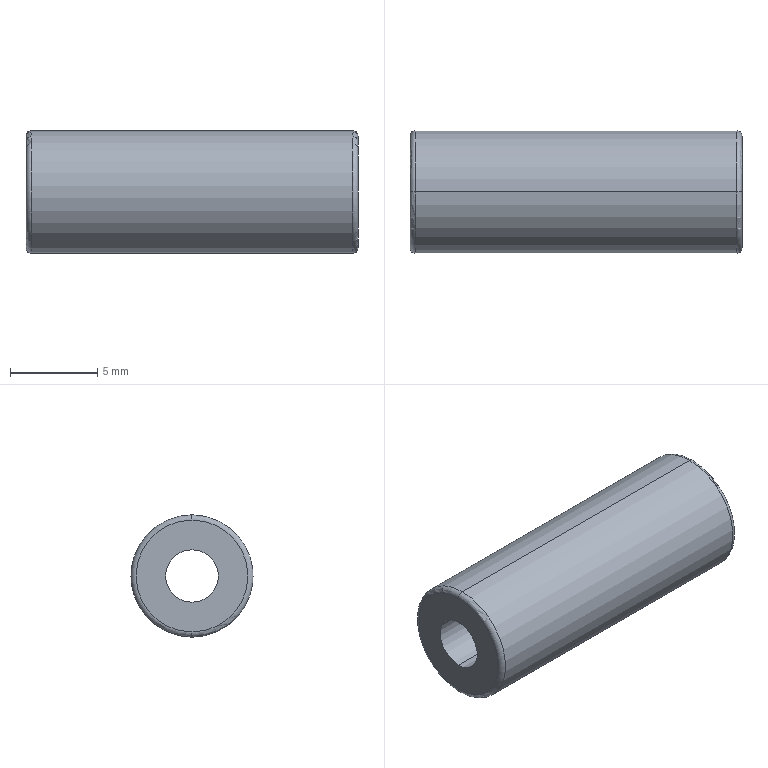Part | SolidWorks | features Revolution 1 | 1 solid | 10 faces | box 19 x 7 x 7 mm | volume 596.069 mm3 | torus 4 | cylinder 4 | plane 2 | commonest cylinder face diameters 3 x2 7 x2
STEP:
#1=CARTESIAN_POINT('',(0.3,0.,3.5));
#2=VERTEX_POINT('',#1);
#3=CARTESIAN_POINT('',(0.3,0.,-3.5));
#4=VERTEX_POINT('',#3);
#5=CARTESIAN_POINT('',(0.3,0.,0.));
#6=DIRECTION('',(-1.,0.,0.));
#7=DIRECTION('',(0.,0.,1.));
#8=AXIS2_PLACEMENT_3D('',#5,#6,#7);
#9=CIRCLE('',#8,3.5);
#10=EDGE_CURVE('',#2,#4,#9,.T.);
#11=ORIENTED_EDGE('',*,*,#10,.T.);
#12=CARTESIAN_POINT('',(0.,0.,-3.2));
#13=VERTEX_POINT('',#12);
#14=CARTESIAN_POINT('',(0.3,0.,-3.2));
#15=DIRECTION('',(0.,1.,0.));
#16=DIRECTION('',(0.,0.,1.));
#17=AXIS2_PLACEMENT_3D('',#14,#15,#16);
#18=CIRCLE('',#17,0.3);
#19=EDGE_CURVE('',#4,#13,#18,.T.);
#20=ORIENTED_EDGE('',*,*,#19,.T.);
#21=CARTESIAN_POINT('',(0.,0.,3.2));
#22=VERTEX_POINT('',#21);
#23=CARTESIAN_POINT('',(0.,0.,0.));
#24=DIRECTION('',(-1.,0.,0.));
#25=DIRECTION('',(0.,0.,1.));
#26=AXIS2_PLACEMENT_3D('',#23,#24,#25);
#27=CIRCLE('',#26,3.2);
#28=EDGE_CURVE('',#22,#13,#27,.T.);
#29=ORIENTED_EDGE('',*,*,#28,.F.);
#30=CARTESIAN_POINT('',(0.3,0.,3.2));
#31=DIRECTION('',(0.,-1.,0.));
#32=DIRECTION('',(0.,0.,-1.));
#33=AXIS2_PLACEMENT_3D('',#30,#31,#32);
#34=CIRCLE('',#33,0.3);
#35=EDGE_CURVE('',#2,#22,#34,.T.);
#36=ORIENTED_EDGE('',*,*,#35,.F.);
#37=EDGE_LOOP('',(#11,#20,#29,#36));
#38=FACE_OUTER_BOUND('',#37,.T.);
#39=CARTESIAN_POINT('',(0.3,0.,0.));
#40=DIRECTION('',(-1.,0.,0.));
#41=DIRECTION('',(0.,0.,1.));
#42=AXIS2_PLACEMENT_3D('',#39,#40,#41);
#43=TOROIDAL_SURFACE('',#42,3.2,0.3);
#44=ADVANCED_FACE('',(#38),#43,.T.);
#45=CARTESIAN_POINT('',(18.7,0.,3.5));
#46=VERTEX_POINT('',#45);
#47=CARTESIAN_POINT('',(18.7,0.,-3.5));
#48=VERTEX_POINT('',#47);
#49=CARTESIAN_POINT('',(18.7,0.,0.));
#50=DIRECTION('',(-1.,0.,0.));
#51=DIRECTION('',(0.,0.,1.));
#52=AXIS2_PLACEMENT_3D('',#49,#50,#51);
#53=CIRCLE('',#52,3.5);
#54=EDGE_CURVE('',#46,#48,#53,.T.);
#55=ORIENTED_EDGE('',*,*,#54,.T.);
#56=CARTESIAN_POINT('',(50.,0.,-3.5));
#57=DIRECTION('',(-1.,0.,0.));
#58=VECTOR('',#57,1000.);
#59=LINE('',#56,#58);
#60=EDGE_CURVE('',#48,#4,#59,.T.);
#61=ORIENTED_EDGE('',*,*,#60,.T.);
#62=ORIENTED_EDGE('',*,*,#10,.F.);
#63=CARTESIAN_POINT('',(50.,0.,3.5));
#64=DIRECTION('',(-1.,0.,0.));
#65=VECTOR('',#64,1000.);
#66=LINE('',#63,#65);
#67=EDGE_CURVE('',#46,#2,#66,.T.);
#68=ORIENTED_EDGE('',*,*,#67,.F.);
#69=EDGE_LOOP('',(#55,#61,#62,#68));
#70=FACE_OUTER_BOUND('',#69,.T.);
#71=CARTESIAN_POINT('',(50.,0.,0.));
#72=DIRECTION('',(-1.,0.,0.));
#73=DIRECTION('',(0.,0.,1.));
#74=AXIS2_PLACEMENT_3D('',#71,#72,#73);
#75=CYLINDRICAL_SURFACE('',#74,3.5);
#76=ADVANCED_FACE('',(#70),#75,.T.);
#77=CARTESIAN_POINT('',(19.,0.,3.2));
#78=VERTEX_POINT('',#77);
#79=CARTESIAN_POINT('',(19.,0.,-3.2));
#80=VERTEX_POINT('',#79);
#81=CARTESIAN_POINT('',(19.,0.,0.));
#82=DIRECTION('',(-1.,0.,0.));
#83=DIRECTION('',(0.,0.,1.));
#84=AXIS2_PLACEMENT_3D('',#81,#82,#83);
#85=CIRCLE('',#84,3.2);
#86=EDGE_CURVE('',#78,#80,#85,.T.);
#87=ORIENTED_EDGE('',*,*,#86,.T.);
#88=CARTESIAN_POINT('',(18.7,0.,-3.2));
#89=DIRECTION('',(0.,1.,0.));
#90=DIRECTION('',(0.,0.,1.));
#91=AXIS2_PLACEMENT_3D('',#88,#89,#90);
#92=CIRCLE('',#91,0.3);
#93=EDGE_CURVE('',#80,#48,#92,.T.);
#94=ORIENTED_EDGE('',*,*,#93,.T.);
#95=ORIENTED_EDGE('',*,*,#54,.F.);
#96=CARTESIAN_POINT('',(18.7,0.,3.2));
#97=DIRECTION('',(0.,-1.,0.));
#98=DIRECTION('',(0.,0.,-1.));
#99=AXIS2_PLACEMENT_3D('',#96,#97,#98);
#100=CIRCLE('',#99,0.3);
#101=EDGE_CURVE('',#78,#46,#100,.T.);
#102=ORIENTED_EDGE('',*,*,#101,.F.);
#103=EDGE_LOOP('',(#87,#94,#95,#102));
#104=FACE_OUTER_BOUND('',#103,.T.);
#105=CARTESIAN_POINT('',(18.7,0.,0.));
#106=DIRECTION('',(-1.,0.,0.));
#107=DIRECTION('',(0.,0.,1.));
#108=AXIS2_PLACEMENT_3D('',#105,#106,#107);
#109=TOROIDAL_SURFACE('',#108,3.2,0.3);
#110=ADVANCED_FACE('',(#104),#109,.T.);
#111=CARTESIAN_POINT('',(19.,0.,-1.5));
#112=VERTEX_POINT('',#111);
#113=CARTESIAN_POINT('',(19.,0.,1.5));
#114=VERTEX_POINT('',#113);
#115=CARTESIAN_POINT('',(19.,0.,0.));
#116=DIRECTION('',(-1.,0.,0.));
#117=DIRECTION('',(0.,0.,1.));
#118=AXIS2_PLACEMENT_3D('',#115,#116,#117);
#119=CIRCLE('',#118,1.5);
#120=EDGE_CURVE('',#112,#114,#119,.T.);
#121=ORIENTED_EDGE('',*,*,#120,.F.);
#122=CARTESIAN_POINT('',(0.,0.,-1.5));
#123=VERTEX_POINT('',#122);
#124=CARTESIAN_POINT('',(50.,0.,-1.5));
#125=DIRECTION('',(-1.,0.,0.));
#126=VECTOR('',#125,1000.);
#127=LINE('',#124,#126);
#128=EDGE_CURVE('',#112,#123,#127,.T.);
#129=ORIENTED_EDGE('',*,*,#128,.T.);
#130=CARTESIAN_POINT('',(0.,0.,1.5));
#131=VERTEX_POINT('',#130);
#132=CARTESIAN_POINT('',(0.,0.,0.));
#133=DIRECTION('',(-1.,0.,0.));
#134=DIRECTION('',(0.,0.,1.));
#135=AXIS2_PLACEMENT_3D('',#132,#133,#134);
#136=CIRCLE('',#135,1.5);
#137=EDGE_CURVE('',#123,#131,#136,.T.);
#138=ORIENTED_EDGE('',*,*,#137,.T.);
#139=CARTESIAN_POINT('',(50.,0.,1.5));
#140=DIRECTION('',(-1.,0.,0.));
#141=VECTOR('',#140,1000.);
#142=LINE('',#139,#141);
#143=EDGE_CURVE('',#114,#131,#142,.T.);
#144=ORIENTED_EDGE('',*,*,#143,.F.);
#145=EDGE_LOOP('',(#121,#129,#138,#144));
#146=FACE_OUTER_BOUND('',#145,.T.);
#147=CARTESIAN_POINT('',(50.,0.,0.));
#148=DIRECTION('',(-1.,0.,0.));
#149=DIRECTION('',(0.,0.,1.));
#150=AXIS2_PLACEMENT_3D('',#147,#148,#149);
#151=CYLINDRICAL_SURFACE('',#150,1.5);
#152=ADVANCED_FACE('',(#146),#151,.F.);
#153=CARTESIAN_POINT('',(0.,0.,0.));
#154=DIRECTION('',(-1.,0.,0.));
#155=DIRECTION('',(0.,0.,1.));
#156=AXIS2_PLACEMENT_3D('',#153,#154,#155);
#157=CIRCLE('',#156,1.5);
#158=EDGE_CURVE('',#131,#123,#157,.T.);
#159=ORIENTED_EDGE('',*,*,#158,.F.);
#160=ORIENTED_EDGE('',*,*,#137,.F.);
#161=EDGE_LOOP('',(#159,#160));
#162=FACE_BOUND('',#161,.T.);
#163=ORIENTED_EDGE('',*,*,#28,.T.);
#164=CARTESIAN_POINT('',(0.,0.,0.));
#165=DIRECTION('',(-1.,0.,0.));
#166=DIRECTION('',(0.,0.,1.));
#167=AXIS2_PLACEMENT_3D('',#164,#165,#166);
#168=CIRCLE('',#167,3.2);
#169=EDGE_CURVE('',#13,#22,#168,.T.);
#170=ORIENTED_EDGE('',*,*,#169,.T.);
#171=EDGE_LOOP('',(#163,#170));
#172=FACE_OUTER_BOUND('',#171,.T.);
#173=CARTESIAN_POINT('',(0.,3.2,0.));
#174=DIRECTION('',(1.,0.,0.));
#175=DIRECTION('',(0.,0.,-1.));
#176=AXIS2_PLACEMENT_3D('',#173,#174,#175);
#177=PLANE('',#176);
#178=ADVANCED_FACE('',(#162,#172),#177,.F.);
#179=ORIENTED_EDGE('',*,*,#128,.F.);
#180=CARTESIAN_POINT('',(19.,0.,0.));
#181=DIRECTION('',(-1.,0.,0.));
#182=DIRECTION('',(0.,0.,1.));
#183=AXIS2_PLACEMENT_3D('',#180,#181,#182);
#184=CIRCLE('',#183,1.5);
#185=EDGE_CURVE('',#114,#112,#184,.T.);
#186=ORIENTED_EDGE('',*,*,#185,.F.);
#187=ORIENTED_EDGE('',*,*,#143,.T.);
#188=ORIENTED_EDGE('',*,*,#158,.T.);
#189=EDGE_LOOP('',(#179,#186,#187,#188));
#190=FACE_OUTER_BOUND('',#189,.T.);
#191=CARTESIAN_POINT('',(50.,0.,0.));
#192=DIRECTION('',(-1.,0.,0.));
#193=DIRECTION('',(0.,0.,1.));
#194=AXIS2_PLACEMENT_3D('',#191,#192,#193);
#195=CYLINDRICAL_SURFACE('',#194,1.5);
#196=ADVANCED_FACE('',(#190),#195,.F.);
#197=ORIENTED_EDGE('',*,*,#86,.F.);
#198=CARTESIAN_POINT('',(19.,0.,0.));
#199=DIRECTION('',(-1.,0.,0.));
#200=DIRECTION('',(0.,0.,1.));
#201=AXIS2_PLACEMENT_3D('',#198,#199,#200);
#202=CIRCLE('',#201,3.2);
#203=EDGE_CURVE('',#80,#78,#202,.T.);
#204=ORIENTED_EDGE('',*,*,#203,.F.);
#205=EDGE_LOOP('',(#197,#204));
#206=FACE_OUTER_BOUND('',#205,.T.);
#207=ORIENTED_EDGE('',*,*,#185,.T.);
#208=ORIENTED_EDGE('',*,*,#120,.T.);
#209=EDGE_LOOP('',(#207,#208));
#210=FACE_BOUND('',#209,.T.);
#211=CARTESIAN_POINT('',(19.,1.5,0.));
#212=DIRECTION('',(-1.,0.,0.));
#213=DIRECTION('',(0.,0.,1.));
#214=AXIS2_PLACEMENT_3D('',#211,#212,#213);
#215=PLANE('',#214);
#216=ADVANCED_FACE('',(#206,#210),#215,.F.);
#217=ORIENTED_EDGE('',*,*,#93,.F.);
#218=ORIENTED_EDGE('',*,*,#203,.T.);
#219=ORIENTED_EDGE('',*,*,#101,.T.);
#220=CARTESIAN_POINT('',(18.7,0.,0.));
#221=DIRECTION('',(-1.,0.,0.));
#222=DIRECTION('',(0.,0.,1.));
#223=AXIS2_PLACEMENT_3D('',#220,#221,#222);
#224=CIRCLE('',#223,3.5);
#225=EDGE_CURVE('',#48,#46,#224,.T.);
#226=ORIENTED_EDGE('',*,*,#225,.F.);
#227=EDGE_LOOP('',(#217,#218,#219,#226));
#228=FACE_OUTER_BOUND('',#227,.T.);
#229=CARTESIAN_POINT('',(18.7,0.,0.));
#230=DIRECTION('',(-1.,0.,0.));
#231=DIRECTION('',(0.,0.,1.));
#232=AXIS2_PLACEMENT_3D('',#229,#230,#231);
#233=TOROIDAL_SURFACE('',#232,3.2,0.3);
#234=ADVANCED_FACE('',(#228),#233,.T.);
#235=ORIENTED_EDGE('',*,*,#60,.F.);
#236=ORIENTED_EDGE('',*,*,#225,.T.);
#237=ORIENTED_EDGE('',*,*,#67,.T.);
#238=CARTESIAN_POINT('',(0.3,0.,0.));
#239=DIRECTION('',(-1.,0.,0.));
#240=DIRECTION('',(0.,0.,1.));
#241=AXIS2_PLACEMENT_3D('',#238,#239,#240);
#242=CIRCLE('',#241,3.5);
#243=EDGE_CURVE('',#4,#2,#242,.T.);
#244=ORIENTED_EDGE('',*,*,#243,.F.);
#245=EDGE_LOOP('',(#235,#236,#237,#244));
#246=FACE_OUTER_BOUND('',#245,.T.);
#247=CARTESIAN_POINT('',(50.,0.,0.));
#248=DIRECTION('',(-1.,0.,0.));
#249=DIRECTION('',(0.,0.,1.));
#250=AXIS2_PLACEMENT_3D('',#247,#248,#249);
#251=CYLINDRICAL_SURFACE('',#250,3.5);
#252=ADVANCED_FACE('',(#246),#251,.T.);
#253=ORIENTED_EDGE('',*,*,#19,.F.);
#254=ORIENTED_EDGE('',*,*,#243,.T.);
#255=ORIENTED_EDGE('',*,*,#35,.T.);
#256=ORIENTED_EDGE('',*,*,#169,.F.);
#257=EDGE_LOOP('',(#253,#254,#255,#256));
#258=FACE_OUTER_BOUND('',#257,.T.);
#259=CARTESIAN_POINT('',(0.3,0.,0.));
#260=DIRECTION('',(-1.,0.,0.));
#261=DIRECTION('',(0.,0.,1.));
#262=AXIS2_PLACEMENT_3D('',#259,#260,#261);
#263=TOROIDAL_SURFACE('',#262,3.2,0.3);
#264=ADVANCED_FACE('',(#258),#263,.T.);
#265=CLOSED_SHELL('',(#44,#76,#110,#152,#178,#196,#216,#234,#252,#264));
#266=MANIFOLD_SOLID_BREP('',#265);
#267=CARTESIAN_POINT('',(0.,0.,0.));
#268=DIRECTION('',(0.,0.,1.));
#269=DIRECTION('',(1.,0.,0.));
#270=AXIS2_PLACEMENT_3D('',#267,#268,#269);
#271=(LENGTH_UNIT()NAMED_UNIT(*)SI_UNIT(.MILLI.,.METRE.));
#272=UNCERTAINTY_MEASURE_WITH_UNIT(LENGTH_MEASURE(0.00001),#271,'','');
#273=(NAMED_UNIT(*)PLANE_ANGLE_UNIT()SI_UNIT($,.RADIAN.));
#274=(NAMED_UNIT(*)SI_UNIT($,.STERADIAN.)SOLID_ANGLE_UNIT());
#275=(GEOMETRIC_REPRESENTATION_CONTEXT(3)GLOBAL_UNCERTAINTY_ASSIGNED_CONTEXT((#272))GLOBAL_UNIT_ASSIGNED_CONTEXT((#271,#273,#274))REPRESENTATION_CONTEXT('',''));
#276=ADVANCED_BREP_SHAPE_REPRESENTATION('',(#266,#270),#275);